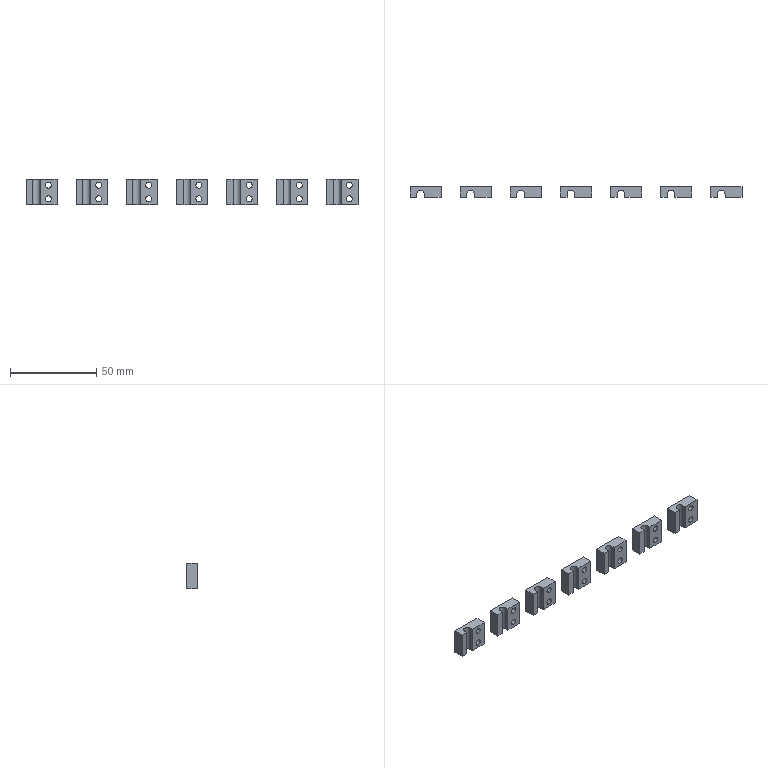NC program | Mastercam | posted with a generic post | part box 192 x 6 x 15 mm
Lines 2657 to 3876 of 12453:
(2 FEM |TOOL - 2|DIA. OFF. - 2|LEN. - 2|TOOL DIA. - 2.)
N5382 T2 M6
N5384 G0 G54 G90 X-65. Y1.856 C0. B0. S7000 M3
N5386 G43 H2 Z50.
N5388 Z3.61
N5390 G1 Z3.11 F600.
N5392 X-64.989 Z2.901 F3000.
N5394 X-64.957 Z2.694
N5396 X-64.902 Z2.492
N5398 X-64.827 Z2.296
N5400 X-64.732 Z2.11
N5402 X-64.618 Z1.934
N5404 X-64.487 Z1.771
N5406 X-64.338 Z1.623
N5408 X-64.176 Z1.492
N5410 X-64. Z1.378
N5412 X-63.814 Z1.283
N5414 X-63.618 Z1.208
N5416 X-63.416 Z1.153
N5418 X-63.209 Z1.121
N5420 X-63. Z1.11
N5422 G2 X-61. Y-.144 Z1. J-2.
N5424 G1 Y-1.244 Z.981
N5426 Y-2.344 Z.962
N5428 Y-3.444 Z.943
N5430 Y-4.544 Z.924
N5432 Y-6.4 Z.905
N5434 Y-5.644
N5436 Y-4.544 Z.886
N5438 Y-3.444 Z.867
N5440 Y-2.344 Z.848
N5442 Y-1.244 Z.83
N5444 Y-.144 Z.811
N5446 Y0. Z.808
N5448 Y.956 Z.792
N5450 Y2.056 Z.773
N5452 Y3.156 Z.754
N5454 Y4.256 Z.735
N5456 Y6.4 Z.716
N5458 Y5.356
N5460 Y4.256 Z.697
N5462 Y3.156 Z.678
N5464 Y2.056 Z.659
N5466 Y.956 Z.64
N5468 Y-.144 Z.621
N5470 Y-1.244 Z.602
N5472 Y-2.344 Z.583
N5474 Y-3.444 Z.564
N5476 Y-4.544 Z.545
N5478 Y-6.4 Z.527
N5480 Y-5.644
N5482 Y-4.544 Z.508
N5484 Y-3.444 Z.489
N5486 Y-2.344 Z.47
N5488 Y-1.244 Z.451
N5490 Y-.144 Z.432
N5492 Y0. Z.429
N5494 Y.956 Z.413
N5496 Y2.056 Z.394
N5498 Y3.156 Z.375
N5500 Y4.256 Z.356
N5502 Y6.4 Z.337
N5504 Y5.356
N5506 Y4.256 Z.318
N5508 Y3.156 Z.299
N5510 Y2.056 Z.28
N5512 Y.956 Z.261
N5514 Y-.144 Z.242
N5516 Y-1.244 Z.223
N5518 Y-2.344 Z.205
N5520 Y-3.444 Z.186
N5522 Y-4.544 Z.167
N5524 Y-6.4 Z.148
N5526 Y-5.644
N5528 Y-4.544 Z.129
N5530 Y-3.444 Z.11
N5532 Y-2.344 Z.091
N5534 Y-1.244 Z.072
N5536 Y-.144 Z.053
N5538 Y0. Z.051
N5540 Y.956 Z.034
N5542 Y2.056 Z.015
N5544 Y3.156 Z-.004
N5546 Y4.256 Z-.023
N5548 Y6.4 Z-.042
N5550 Y5.356
N5552 Y4.256 Z-.061
N5554 Y3.156 Z-.08
N5556 Y2.056 Z-.098
N5558 Y.956 Z-.117
N5560 Y-.144 Z-.136
N5562 Y-1.244 Z-.155
N5564 Y-2.344 Z-.174
N5566 Y-3.444 Z-.193
N5568 Y-4.544 Z-.212
N5570 Y-6.4 Z-.231
N5572 Y-5.644
N5574 Y-4.544 Z-.25
N5576 Y0.
N5578 Y6.4
N5580 Y-6.4
N5582 Y-4.544
N5584 G2 X-60.849 Y-4.346 I.206
N5586 G1 X-60.051 Y-4.124
N5588 G3 X-59.9 Y-3.926 I-.055 J.198
N5590 G1 Y0.
N5592 Y7.5
N5594 X-62.1
N5596 Y-7.5
N5598 X-59.9
N5600 Y-3.926
N5602 G3 X-59.902 Y-3.894 I-.206
N5604 G1 X-60.997 Y3.262
N5606 G2 X-61. Y3.293 I.203 J.031
N5608 G1 Y4.393 Z-.268
N5610 Y6.4 Z-.286
N5612 Y5.493
N5614 Y4.393 Z-.304
N5616 Y3.293 Z-.321
N5618 Y2.193 Z-.339
N5620 Y1.093 Z-.357
N5622 Y-.007 Z-.375
N5624 Y-1.107 Z-.393
N5626 Y-2.207 Z-.411
N5628 Y-3.307 Z-.429
N5630 Y-4.407 Z-.446
N5632 Y-6.4 Z-.464
N5634 Y-5.507
N5636 Y-4.407 Z-.482
N5638 Y-3.307 Z-.5
N5640 Y0.
N5642 Y6.4
N5644 Y-6.4
N5646 Y-3.307
N5648 G2 X-60.849 Y-3.108 I.206
N5650 G1 X-60.051 Y-2.887
N5652 G3 X-59.9 Y-2.688 I-.055 J.199
N5654 G1 Y0.
N5656 Y7.5
N5658 X-62.1
N5660 Y-7.5
N5662 X-59.9
N5664 Y-2.688
N5666 G3 X-59.902 Y-2.657 I-.206
N5668 G1 X-60.997 Y4.499
N5670 G2 X-61. Y4.531 I.203 J.032
N5672 G1 Y6.4 Z-.518
N5674 Y5.631
N5676 Y4.531 Z-.536
N5678 Y3.431 Z-.554
N5680 Y2.331 Z-.571
N5682 Y1.231 Z-.589
N5684 Y.131 Z-.607
N5686 Y-.969 Z-.625
N5688 Y-2.069 Z-.643
N5690 Y-3.169 Z-.661
N5692 Y-4.269 Z-.679
N5694 Y-6.4 Z-.696
N5696 Y-5.369
N5698 Y-4.269 Z-.714
N5700 Y-3.169 Z-.732
N5702 Y-2.069 Z-.75
N5704 Y0.
N5706 Y6.4
N5708 Y-6.4
N5710 Y-2.069
N5712 G2 X-60.849 Y-1.871 I.206
N5714 G1 X-60.051 Y-1.649
N5716 G3 X-59.9 Y-1.451 I-.055 J.198
N5718 G1 Y0.
N5720 Y7.5
N5722 X-62.1
N5724 Y-7.5
N5726 X-59.9
N5728 Y-1.451
N5730 G3 X-59.902 Y-1.423 I-.206
N5732 G1 X-60.59 Y3.596
N5734 G3 X-60.794 Y3.774 I-.204 J-.028
N5736 X-61. Y3.568 J-.206
N5738 G1 Y2.468 Z-.768
N5740 Y1.368 Z-.786
N5742 Y.268 Z-.804
N5744 Y-.832 Z-.821
N5746 Y-1.932 Z-.839
N5748 Y-3.032 Z-.857
N5750 Y-4.132 Z-.875
N5752 Y-5.232 Z-.893
N5754 Y-6.4 Z-.911
N5756 Y-6.332
N5758 Y-5.232 Z-.929
N5760 Y-4.132 Z-.946
N5762 Y-3.032 Z-.964
N5764 Y-1.932 Z-.982
N5766 Y-.832 Z-1.
N5768 Y0.
N5770 Y6.4
N5772 Y-6.4
N5774 Y-.832
N5776 G2 X-60.849 Y-.633 I.206
N5778 G1 X-60.051 Y-.412
N5780 G3 X-59.9 Y-.213 I-.055 J.199
N5782 G1 Y0.
N5784 Y7.5
N5786 X-62.1
N5788 Y-7.5
N5790 X-59.9
N5792 Y-.213
N5794 G3 X-59.902 Y-.183 I-.206
N5796 G1 X-60.59 Y4.43
N5798 G3 X-60.794 Y4.606 I-.204 J-.03
N5800 X-61. Y4.4 J-.206
N5802 G1 Y3.3 Z-1.018
N5804 Y2.2 Z-1.036
N5806 Y1.1 Z-1.054
N5808 Y0. Z-1.071
N5810 Y-1.1 Z-1.089
N5812 Y-2.2 Z-1.107
N5814 Y-3.3 Z-1.125
N5816 Y-4.4 Z-1.143
N5818 Y-6.4 Z-1.161
N5820 Y-5.5
N5822 Y-4.4 Z-1.179
N5824 Y-3.3 Z-1.196
N5826 Y-2.2 Z-1.214
N5828 Y-1.1 Z-1.232
N5830 Y0. Z-1.25
N5832 Y6.4
N5834 Y-6.4
N5836 Y0.
N5838 G2 X-60.849 Y.199 I.206
N5840 G1 X-60.051 Y.42
N5842 G3 X-59.9 Y.619 I-.055 J.199
N5844 G1 Y7.5
N5846 X-62.1
N5848 Y-7.5
N5850 X-59.9
N5852 Y0.
N5854 Y.619
N5856 G3 X-59.906 Y.668 I-.206
N5858 G1 X-60.594 Y3.486
N5860 G3 X-60.794 Y3.643 I-.2 J-.049
N5862 X-61. Y3.437 J-.206
N5864 G1 Y2.337 Z-1.268
N5866 Y1.237 Z-1.286
N5868 Y.137 Z-1.304
N5870 Y-.963 Z-1.321
N5872 Y-2.063 Z-1.339
N5874 Y-3.163 Z-1.357
N5876 Y-4.263 Z-1.375
N5878 Y-6.4 Z-1.393
N5880 Y-5.362
N5882 Y-4.263 Z-1.411
N5884 Y-3.163 Z-1.429
N5886 Y-2.063 Z-1.446
N5888 Y-.963 Z-1.464
N5890 Y0. Z-1.48
N5892 Y.138 Z-1.482
N5894 Y1.238 Z-1.5
N5896 Y6.4
N5898 Y-6.4
N5900 Y0.
N5902 Y1.238
N5904 G2 X-60.849 Y1.436 I.206
N5906 G1 X-60.051 Y1.657
N5908 G3 X-59.9 Y1.856 I-.055 J.199
N5910 G1 Y7.5
N5912 X-62.1
N5914 Y-7.5
N5916 X-59.9
N5918 Y0.
N5920 Y1.856
N5922 G3 X-60.106 Y2.062 I-.206
N5924 X-60.295 Y1.939 J-.206
N5926 G1 X-60.983 Y.357
N5928 G3 X-61. Y.275 I.189 J-.082
N5930 G1 Y-.825 Z-1.518
N5932 Y-1.925 Z-1.536
N5934 Y-3.025 Z-1.554
N5936 Y-4.125 Z-1.571
N5938 Y-5.225 Z-1.589
N5940 Y-6.4 Z-1.607
N5942 Y-6.325
N5944 Y-5.225 Z-1.625
N5946 Y-4.125 Z-1.643
N5948 Y-3.025 Z-1.661
N5950 Y-1.925 Z-1.679
N5952 Y-.825 Z-1.696
N5954 Y0. Z-1.71
N5956 Y.275 Z-1.714
N5958 Y1.375 Z-1.732
N5960 Y2.475 Z-1.75
N5962 Y6.4
N5964 Y-6.4
N5966 Y0.
N5968 Y2.475
N5970 G2 X-60.849 Y2.674 I.206
N5972 G1 X-60.051 Y2.895
N5974 G3 X-59.9 Y3.094 I-.055 J.199
N5976 G1 Y7.5
N5978 X-62.1
N5980 Y-7.5
N5982 X-59.9
N5984 Y0.
N5986 Y3.094
N5988 G3 X-60.106 Y3.3 I-.206
N5990 X-60.309 Y3.131 J-.206
N5992 G1 X-60.997 Y-.651
N5994 G3 X-61. Y-.688 I.203 J-.037
N5996 G1 Y-1.788 Z-1.768
N5998 Y-2.888 Z-1.786
N6000 Y-3.988 Z-1.804
N6002 Y-5.088 Z-1.821
N6004 Y-6.42 Z-1.839
N6006 Y-6.188
N6008 Y-5.088 Z-1.857
N6010 Y-3.988 Z-1.875
N6012 Y-2.888 Z-1.893
N6014 Y-1.788 Z-1.911
N6016 Y-.688 Z-1.929
N6018 Y.412 Z-1.946
N6020 Y1.512 Z-1.964
N6022 Y2.612 Z-1.982
N6024 Y3.712 Z-2.
N6026 Y6.42
N6028 Y0.
N6030 Y-6.42
N6032 Y3.712
N6034 G2 X-60.85 Y3.911 I.206
N6036 G1 X-60.07 Y4.133
N6038 G3 X-59.92 Y4.331 I-.056 J.198
N6040 G1 Y7.5
N6042 X-62.08
N6044 Y0.
N6046 Y-7.5
N6048 X-59.92
N6050 Y4.331
N6052 G3 X-60.126 Y4.537 I-.206
N6054 X-60.331 Y4.354 J-.206
N6056 G1 X-60.999 Y-1.627
N6058 G3 X-61. Y-1.65 I.205 J-.023
N6060 G1 Y-2.75 Z-2.018
N6062 Y-3.85 Z-2.036
N6064 Y-4.95 Z-2.054
N6066 Y-6.453 Z-2.071
N6068 Y-6.05
N6070 Y-4.95 Z-2.089
N6072 Y-3.85 Z-2.107
N6074 Y-2.75 Z-2.125
N6076 Y-1.65 Z-2.143
N6078 Y-.55 Z-2.161
N6080 Y0. Z-2.17
N6082 Y.55 Z-2.179
N6084 Y1.65 Z-2.196
N6086 Y2.75 Z-2.214
N6088 Y3.85 Z-2.232
N6090 Y4.95 Z-2.25
N6092 Y6.453
N6094 Y-6.453
N6096 Y0.
N6098 Y4.95
N6100 G2 X-60.852 Y5.148 I.206
N6102 G1 X-60.101 Y5.371
N6104 G3 X-59.953 Y5.569 I-.058 J.198
N6106 G1 Y7.5
N6108 X-62.047
N6110 Y-7.5
N6112 X-59.953
N6114 Y0.
N6116 Y5.569
N6118 G3 X-60.151 Y5.775 I-.206
N6120 G1 X-60.159
N6122 G3 X-60.365 Y5.585 J-.206
N6124 G1 X-61. Y-2.597
N6126 Y-2.613
N6128 Y-3.713 Z-2.268
N6130 Y-4.813 Z-2.286
N6132 Y-6.529 Z-2.304
N6134 Y-5.913
N6136 Y-4.813 Z-2.321
N6138 Y-3.713 Z-2.339
N6140 Y-2.613 Z-2.357
N6142 Y-1.513 Z-2.375
N6144 Y-.413 Z-2.393
N6146 Y0. Z-2.4
N6148 Y.687 Z-2.411
N6150 Y1.787 Z-2.429
N6152 Y2.887 Z-2.446
N6154 Y3.987 Z-2.464
N6156 Y5.087 Z-2.482
N6158 Y6.187 Z-2.5
N6160 Y6.529
N6162 Y-6.529
N6164 Y0.
N6166 Y6.187
N6168 G2 X-60.858 Y6.383 I.206
N6170 G1 X-60.17 Y6.61
N6172 G3 X-60.029 Y6.806 I-.065 J.196
N6174 G1 Y7.5
N6176 X-61.971
N6178 Y-7.5
N6180 X-60.029
N6182 Y0.
N6184 Y6.806
N6186 G3 X-60.128 Y6.909 I-.103
N6188 G1 X-60.132
N6190 G3 X-60.235 Y6.814 J-.103
N6192 G1 X-61. Y-2.763
N6194 Y-2.779
N6196 Y-3.879 Z-2.518
N6198 Y-4.979 Z-2.536
N6200 Y-6.639 Z-2.554
N6202 Y-6.079
N6204 Y-4.979 Z-2.571
N6206 Y-3.879 Z-2.589
N6208 Y-2.779 Z-2.607
N6210 Y-1.679 Z-2.625
N6212 Y-.579 Z-2.643
N6214 Y0. Z-2.652
N6216 Y.521 Z-2.661
N6218 Y1.621 Z-2.679
N6220 Y2.721 Z-2.696
N6222 Y3.821 Z-2.714
N6224 Y4.921 Z-2.732
N6226 Y6.639 Z-2.75
N6228 Y6.021
N6230 Y-6.639
N6232 Y0.
N6234 Y6.639
N6236 Y6.021
N6238 G2 X-61.131 Y5.828 I-.206
N6240 G1 X-61.73 Y5.594
N6242 G3 X-61.861 Y5.402 I.075 J-.192
N6244 G1 Y-7.5
N6246 X-60.139
N6248 Y0.
N6250 Y7.5
N6252 X-61.861
N6254 Y5.402
N6256 Y5.193 Z-2.739
N6258 Y4.986 Z-2.706
N6260 Y4.784 Z-2.652
N6262 Y4.588 Z-2.577
N6264 Y4.402 Z-2.482
N6266 Y4.226 Z-2.368
N6268 Y4.064 Z-2.236
N6270 Y3.916 Z-2.088
N6272 Y3.784 Z-1.926
N6274 Y3.67 Z-1.75
N6276 Y3.575 Z-1.563
N6278 Y3.5 Z-1.368
N6280 Y3.445 Z-1.166
N6282 Y3.413 Z-.959
N6284 Y3.402 Z-.75
N6286 Z-.25
N6288 G0 Z50.
N6290 X-60.282 Y-6.465
N6292 Z-.25
N6294 G1 Z-.75 F600.
N6296 Y-6.454 Z-.957 F3000.
N6298 Y-6.422 Z-1.162
N6300 Y-6.369 Z-1.362
N6302 Y-6.296 Z-1.556
N6304 Y-6.202 Z-1.741
N6306 Y-6.091 Z-1.915
N6308 Y-5.961 Z-2.077
N6310 Y-5.816 Z-2.225
N6312 Y-5.656 Z-2.357
N6314 Y-5.484 Z-2.471
N6316 Y-5.3 Z-2.568
N6318 Y-5.108 Z-2.644
N6320 Y-4.908 Z-2.701
N6322 Y-4.704 Z-2.736
N6324 Y-4.498 Z-2.75
N6326 Y-3.398 Z-2.768
N6328 Y-2.298 Z-2.786
N6330 Y-1.198 Z-2.804
N6332 Y-.098 Z-2.821
N6334 Y1.002 Z-2.839
N6336 Y2.102 Z-2.857
N6338 Y3.202 Z-2.875
N6340 Y4.302 Z-2.893
N6342 Y5.402 Z-2.911
N6344 Y6.502 Z-2.929
N6346 Y7.5 Z-2.945
N6348 X-60.747 Z-2.946
N6350 X-61.718 Z-2.962
N6352 Y6.983 Z-2.964
N6354 Y5.883 Z-2.982
N6356 Y4.783 Z-3.
N6358 Y0.
N6360 Y-7.5
N6362 X-60.282
N6364 Y7.5
N6366 X-61.718
N6368 Y4.783
N6370 G3 X-61.717 Y4.764 I.206
N6372 G1 X-60.899 Y-3.952
N6374 G3 X-60.693 Y-4.139 I.206 J.02
N6376 G1 X-60.684
N6378 G3 X-60.487 Y-3.932 I-.009 J.206
N6380 G1 Y-2.832 Z-3.018
N6382 Y-1.732 Z-3.036
N6384 Y-.632 Z-3.054
N6386 Y.468 Z-3.071
N6388 Y1.568 Z-3.089
N6390 Y2.668 Z-3.107
N6392 Y3.768 Z-3.125
N6394 Y4.868 Z-3.143
N6396 Y5.968 Z-3.161
N6398 Y7.068 Z-3.179
N6400 Y7.5 Z-3.186
N6402 X-61.513 Z-3.196
N6404 Y7.464
N6406 Y6.364 Z-3.214
N6408 Y5.264 Z-3.232
N6410 Y4.164 Z-3.25
N6412 Y0.
N6414 Y-7.5
N6416 X-60.487
N6418 Y7.5
N6420 X-61.513
N6422 Y4.164
N6424 Y4.157
N6426 X-61.19 Y-5.168
N6428 G3 X-60.984 Y-5.367 I.206 J.007
N6430 G1 X-60.98
N6432 G3 X-60.778 Y-5.161 I-.004 J.206
N6434 G1 Y-4.061 Z-3.268
N6436 Y-2.961 Z-3.286
N6438 Y-1.861 Z-3.304
N6440 Y-.761 Z-3.321
N6442 Y0. Z-3.334
N6444 Y.339 Z-3.339
N6446 Y1.439 Z-3.357
N6448 Y2.539 Z-3.375
N6450 Y3.639 Z-3.393
N6452 Y4.739 Z-3.411
N6454 Y5.839 Z-3.429
N6456 Y7.5 Z-3.446
N6458 X-61.222
N6460 Y6.846
N6462 Y5.746 Z-3.464
N6464 Y4.646 Z-3.482
N6466 Y3.546 Z-3.5
N6468 Y-7.443
N6470 Y-7.5
N6472 X-60.778
N6474 Y0.
N6476 Y7.5
N6478 X-61.222
N6480 Y3.546
N6482 Y3.336 Z-3.489
N6484 Y3.13 Z-3.456
N6486 Y2.928 Z-3.402
N6488 Y2.732 Z-3.327
N6490 Y2.546 Z-3.232
N6492 Y2.37 Z-3.118
N6494 Y2.207 Z-2.986
N6496 Y2.059 Z-2.838
N6498 Y1.928 Z-2.676
N6500 Y1.813 Z-2.5
N6502 Y1.718 Z-2.313
N6504 Y1.643 Z-2.118
N6506 Y1.589 Z-1.916
N6508 Y1.557 Z-1.709
N6510 Y1.546 Z-1.5
N6512 Z-1.
N6514 G0 Z50.
N6516 X-36. Y1.856
N6518 Z3.61
N6520 G1 Z3.11 F600.
N6522 X-35.989 Z2.901 F3000.
N6524 X-35.957 Z2.694
N6526 X-35.902 Z2.492
N6528 X-35.827 Z2.296
N6530 X-35.732 Z2.11
N6532 X-35.618 Z1.934
N6534 X-35.487 Z1.771
N6536 X-35.338 Z1.623
N6538 X-35.176 Z1.492
N6540 X-35. Z1.378
N6542 X-34.814 Z1.283
N6544 X-34.618 Z1.208
N6546 X-34.416 Z1.153
N6548 X-34.209 Z1.121
N6550 X-34. Z1.11
N6552 G2 X-32. Y-.144 Z1. J-2.
N6554 G1 Y-1.244 Z.981
N6556 Y-2.344 Z.962
N6558 Y-3.444 Z.943
N6560 Y-4.544 Z.924
N6562 Y-6.4 Z.905
N6564 Y-5.644
N6566 Y-4.544 Z.886
N6568 Y-3.444 Z.867
N6570 Y-2.344 Z.848
N6572 Y-1.244 Z.83
N6574 Y-.144 Z.811
N6576 Y0. Z.808
N6578 Y.956 Z.792
N6580 Y2.056 Z.773
N6582 Y3.156 Z.754
N6584 Y4.256 Z.735
N6586 Y6.4 Z.716
N6588 Y5.356
N6590 Y4.256 Z.697
N6592 Y3.156 Z.678
N6594 Y2.056 Z.659
N6596 Y.956 Z.64
N6598 Y-.144 Z.621
N6600 Y-1.244 Z.602
N6602 Y-2.344 Z.583
N6604 Y-3.444 Z.564
N6606 Y-4.544 Z.545
N6608 Y-6.4 Z.527
N6610 Y-5.644
N6612 Y-4.544 Z.508
N6614 Y-3.444 Z.489
N6616 Y-2.344 Z.47
N6618 Y-1.244 Z.451
N6620 Y-.144 Z.432
N6622 Y0. Z.429
N6624 Y.956 Z.413
N6626 Y2.056 Z.394
N6628 Y3.156 Z.375
N6630 Y4.256 Z.356
N6632 Y6.4 Z.337
N6634 Y5.356
N6636 Y4.256 Z.318
N6638 Y3.156 Z.299
N6640 Y2.056 Z.28
N6642 Y.956 Z.261
N6644 Y-.144 Z.242
N6646 Y-1.244 Z.223
N6648 Y-2.344 Z.205
N6650 Y-3.444 Z.186
N6652 Y-4.544 Z.167
N6654 Y-6.4 Z.148
N6656 Y-5.644
N6658 Y-4.544 Z.129
N6660 Y-3.444 Z.11
N6662 Y-2.344 Z.091
N6664 Y-1.244 Z.072
N6666 Y-.144 Z.053
N6668 Y0. Z.051
N6670 Y.956 Z.034
N6672 Y2.056 Z.015
N6674 Y3.156 Z-.004
N6676 Y4.256 Z-.023
N6678 Y6.4 Z-.042
N6680 Y5.356
N6682 Y4.256 Z-.061
N6684 Y3.156 Z-.08
N6686 Y2.056 Z-.098
N6688 Y.956 Z-.117
N6690 Y-.144 Z-.136
N6692 Y-1.244 Z-.155
N6694 Y-2.344 Z-.174
N6696 Y-3.444 Z-.193
N6698 Y-4.544 Z-.212
N6700 Y-6.4 Z-.231
N6702 Y-5.644
N6704 Y-4.544 Z-.25
N6706 Y0.
N6708 Y6.4
N6710 Y-6.4
N6712 Y-4.544
N6714 G2 X-31.849 Y-4.346 I.206
N6716 G1 X-31.051 Y-4.124
N6718 G3 X-30.9 Y-3.926 I-.055 J.198
N6720 G1 Y0.
N6722 Y7.5
N6724 X-33.1
N6726 Y-7.5
N6728 X-30.9
N6730 Y-3.926
N6732 G3 X-30.902 Y-3.894 I-.206
N6734 G1 X-31.997 Y3.262
N6736 G2 X-32. Y3.293 I.203 J.031
N6738 G1 Y4.393 Z-.268
N6740 Y6.4 Z-.286
N6742 Y5.493
N6744 Y4.393 Z-.304
N6746 Y3.293 Z-.321
N6748 Y2.193 Z-.339
N6750 Y1.093 Z-.357
N6752 Y-.007 Z-.375
N6754 Y-1.107 Z-.393
N6756 Y-2.207 Z-.411
N6758 Y-3.307 Z-.429
N6760 Y-4.407 Z-.446
N6762 Y-6.4 Z-.464
N6764 Y-5.507
N6766 Y-4.407 Z-.482
N6768 Y-3.307 Z-.5
N6770 Y0.
N6772 Y6.4
N6774 Y-6.4
N6776 Y-3.307
N6778 G2 X-31.849 Y-3.108 I.206
N6780 G1 X-31.051 Y-2.887
N6782 G3 X-30.9 Y-2.688 I-.055 J.199
N6784 G1 Y0.
N6786 Y7.5
N6788 X-33.1
N6790 Y-7.5
N6792 X-30.9
N6794 Y-2.688
N6796 G3 X-30.902 Y-2.657 I-.206
N6798 G1 X-31.997 Y4.499
N6800 G2 X-32. Y4.531 I.203 J.032
N6802 G1 Y6.4 Z-.518
N6804 Y5.631
N6806 Y4.531 Z-.536
N6808 Y3.431 Z-.554
N6810 Y2.331 Z-.571
N6812 Y1.231 Z-.589
N6814 Y.131 Z-.607
N6816 Y-.969 Z-.625
N6818 Y-2.069 Z-.643
N6820 Y-3.169 Z-.661
N6822 Y-4.269 Z-.679
N6824 Y-6.4 Z-.696
N6826 Y-5.369
N6828 Y-4.269 Z-.714
N6830 Y-3.169 Z-.732
N6832 Y-2.069 Z-.75
N6834 Y0.
N6836 Y6.4
N6838 Y-6.4
N6840 Y-2.069
N6842 G2 X-31.849 Y-1.871 I.206
N6844 G1 X-31.051 Y-1.649
N6846 G3 X-30.9 Y-1.451 I-.055 J.198
N6848 G1 Y0.
N6850 Y7.5
N6852 X-33.1
N6854 Y-7.5
N6856 X-30.9
N6858 Y-1.451
N6860 G3 X-30.902 Y-1.423 I-.206
N6862 G1 X-31.59 Y3.596
N6864 G3 X-31.794 Y3.774 I-.204 J-.028
N6866 X-32. Y3.568 J-.206
N6868 G1 Y2.468 Z-.768
N6870 Y1.368 Z-.786
N6872 Y.268 Z-.804
N6874 Y-.832 Z-.821
N6876 Y-1.932 Z-.839
N6878 Y-3.032 Z-.857
N6880 Y-4.132 Z-.875
N6882 Y-5.232 Z-.893
N6884 Y-6.4 Z-.911
N6886 Y-6.332
N6888 Y-5.232 Z-.929
N6890 Y-4.132 Z-.946
N6892 Y-3.032 Z-.964
N6894 Y-1.932 Z-.982
N6896 Y-.832 Z-1.
N6898 Y0.
N6900 Y6.4
N6902 Y-6.4
N6904 Y-.832
N6906 G2 X-31.849 Y-.633 I.206
N6908 G1 X-31.051 Y-.412
N6910 G3 X-30.9 Y-.213 I-.055 J.199
N6912 G1 Y0.
N6914 Y7.5
N6916 X-33.1
N6918 Y-7.5
N6920 X-30.9
N6922 Y-.213
N6924 G3 X-30.902 Y-.183 I-.206
N6926 G1 X-31.59 Y4.43
N6928 G3 X-31.794 Y4.606 I-.204 J-.03
N6930 X-32. Y4.4 J-.206
N6932 G1 Y3.3 Z-1.018
N6934 Y2.2 Z-1.036
N6936 Y1.1 Z-1.054
N6938 Y0. Z-1.071
N6940 Y-1.1 Z-1.089
N6942 Y-2.2 Z-1.107
N6944 Y-3.3 Z-1.125
N6946 Y-4.4 Z-1.143
N6948 Y-6.4 Z-1.161
N6950 Y-5.5
N6952 Y-4.4 Z-1.179
N6954 Y-3.3 Z-1.196
N6956 Y-2.2 Z-1.214
N6958 Y-1.1 Z-1.232
N6960 Y0. Z-1.25
N6962 Y6.4
N6964 Y-6.4
N6966 Y0.
N6968 G2 X-31.849 Y.199 I.206
N6970 G1 X-31.051 Y.42
N6972 G3 X-30.9 Y.619 I-.055 J.199
N6974 G1 Y7.5
N6976 X-33.1
N6978 Y-7.5
N6980 X-30.9
N6982 Y0.
N6984 Y.619
N6986 G3 X-30.906 Y.668 I-.206
N6988 G1 X-31.594 Y3.486
N6990 G3 X-31.794 Y3.643 I-.2 J-.049
N6992 X-32. Y3.437 J-.206
N6994 G1 Y2.337 Z-1.268
N6996 Y1.237 Z-1.286
N6998 Y.137 Z-1.304
N7000 Y-.963 Z-1.321
N7002 Y-2.063 Z-1.339
N7004 Y-3.163 Z-1.357
N7006 Y-4.263 Z-1.375
N7008 Y-6.4 Z-1.393
N7010 Y-5.362
N7012 Y-4.263 Z-1.411
N7014 Y-3.163 Z-1.429
N7016 Y-2.063 Z-1.446
N7018 Y-.963 Z-1.464
N7020 Y0. Z-1.48
N7022 Y.138 Z-1.482
N7024 Y1.238 Z-1.5
N7026 Y6.4
N7028 Y-6.4
N7030 Y0.
N7032 Y1.238
N7034 G2 X-31.849 Y1.436 I.206
N7036 G1 X-31.051 Y1.657
N7038 G3 X-30.9 Y1.856 I-.055 J.199
N7040 G1 Y7.5
N7042 X-33.1
N7044 Y-7.5
N7046 X-30.9
N7048 Y0.
N7050 Y1.856
N7052 G3 X-31.106 Y2.062 I-.206
N7054 X-31.295 Y1.939 J-.206
N7056 G1 X-31.983 Y.357
N7058 G3 X-32. Y.275 I.189 J-.082
N7060 G1 Y-.825 Z-1.518
N7062 Y-1.925 Z-1.536
N7064 Y-3.025 Z-1.554
N7066 Y-4.125 Z-1.571
N7068 Y-5.225 Z-1.589
N7070 Y-6.4 Z-1.607
N7072 Y-6.325
N7074 Y-5.225 Z-1.625
N7076 Y-4.125 Z-1.643
N7078 Y-3.025 Z-1.661
N7080 Y-1.925 Z-1.679
N7082 Y-.825 Z-1.696
N7084 Y0. Z-1.71
N7086 Y.275 Z-1.714
N7088 Y1.375 Z-1.732
N7090 Y2.475 Z-1.75
N7092 Y6.4
N7094 Y-6.4
N7096 Y0.
N7098 Y2.475
N7100 G2 X-31.849 Y2.674 I.206
N7102 G1 X-31.051 Y2.895
N7104 G3 X-30.9 Y3.094 I-.055 J.199
N7106 G1 Y7.5
N7108 X-33.1
N7110 Y-7.5
N7112 X-30.9
N7114 Y0.
N7116 Y3.094
N7118 G3 X-31.106 Y3.3 I-.206
N7120 X-31.309 Y3.131 J-.206
N7122 G1 X-31.997 Y-.651
N7124 G3 X-32. Y-.688 I.203 J-.037
N7126 G1 Y-1.788 Z-1.768
N7128 Y-2.888 Z-1.786
N7130 Y-3.988 Z-1.804
N7132 Y-5.088 Z-1.821
N7134 Y-6.42 Z-1.839
N7136 Y-6.188
N7138 Y-5.088 Z-1.857
N7140 Y-3.988 Z-1.875
N7142 Y-2.888 Z-1.893
N7144 Y-1.788 Z-1.911
N7146 Y-.688 Z-1.929
N7148 Y.412 Z-1.946
N7150 Y1.512 Z-1.964
N7152 Y2.612 Z-1.982
N7154 Y3.712 Z-2.
N7156 Y6.42
N7158 Y0.
N7160 Y-6.42
N7162 Y3.712
N7164 G2 X-31.85 Y3.911 I.206
N7166 G1 X-31.07 Y4.133
N7168 G3 X-30.92 Y4.331 I-.056 J.198
N7170 G1 Y7.5
N7172 X-33.08
N7174 Y0.
N7176 Y-7.5
N7178 X-30.92
N7180 Y4.331
N7182 G3 X-31.126 Y4.537 I-.206
N7184 X-31.331 Y4.354 J-.206
N7186 G1 X-31.999 Y-1.627
N7188 G3 X-32. Y-1.65 I.205 J-.023
N7190 G1 Y-2.75 Z-2.018
N7192 Y-3.85 Z-2.036
N7194 Y-4.95 Z-2.054
N7196 Y-6.453 Z-2.071
N7198 Y-6.05
N7200 Y-4.95 Z-2.089
N7202 Y-3.85 Z-2.107
N7204 Y-2.75 Z-2.125
N7206 Y-1.65 Z-2.143
N7208 Y-.55 Z-2.161
N7210 Y0. Z-2.17
N7212 Y.55 Z-2.179
N7214 Y1.65 Z-2.196
N7216 Y2.75 Z-2.214
N7218 Y3.85 Z-2.232
N7220 Y4.95 Z-2.25
N7222 Y6.453
N7224 Y-6.453
N7226 Y0.
N7228 Y4.95
N7230 G2 X-31.852 Y5.148 I.206
N7232 G1 X-31.101 Y5.371
N7234 G3 X-30.953 Y5.569 I-.058 J.198
N7236 G1 Y7.5
N7238 X-33.047
N7240 Y-7.5
N7242 X-30.953
N7244 Y0.
N7246 Y5.569
N7248 G3 X-31.151 Y5.775 I-.206
N7250 G1 X-31.159
N7252 G3 X-31.365 Y5.585 J-.206
N7254 G1 X-32. Y-2.597
N7256 Y-2.613
N7258 Y-3.713 Z-2.268
N7260 Y-4.813 Z-2.286
N7262 Y-6.529 Z-2.304
N7264 Y-5.913
N7266 Y-4.813 Z-2.321
N7268 Y-3.713 Z-2.339
N7270 Y-2.613 Z-2.357
N7272 Y-1.513 Z-2.375
N7274 Y-.413 Z-2.393
N7276 Y0. Z-2.4
N7278 Y.687 Z-2.411
N7280 Y1.787 Z-2.429
N7282 Y2.887 Z-2.446
N7284 Y3.987 Z-2.464
N7286 Y5.087 Z-2.482
N7288 Y6.187 Z-2.5
N7290 Y6.529
N7292 Y-6.529
N7294 Y0.
N7296 Y6.187
N7298 G2 X-31.858 Y6.383 I.206
N7300 G1 X-31.17 Y6.61
N7302 G3 X-31.029 Y6.806 I-.065 J.196
N7304 G1 Y7.5
N7306 X-32.971
N7308 Y-7.5
N7310 X-31.029
N7312 Y0.
N7314 Y6.806
N7316 G3 X-31.128 Y6.909 I-.103
N7318 G1 X-31.132
N7320 G3 X-31.235 Y6.814 J-.103
N7322 G1 X-32. Y-2.763
N7324 Y-2.779
N7326 Y-3.879 Z-2.518
N7328 Y-4.979 Z-2.536
N7330 Y-6.639 Z-2.554
N7332 Y-6.079
N7334 Y-4.979 Z-2.571
N7336 Y-3.879 Z-2.589
N7338 Y-2.779 Z-2.607
N7340 Y-1.679 Z-2.625
N7342 Y-.579 Z-2.643
N7344 Y0. Z-2.652
N7346 Y.521 Z-2.661
N7348 Y1.621 Z-2.679
N7350 Y2.721 Z-2.696
N7352 Y3.821 Z-2.714
N7354 Y4.921 Z-2.732
N7356 Y6.639 Z-2.75
N7358 Y6.021
N7360 Y-6.639
N7362 Y0.
N7364 Y6.639
N7366 Y6.021
N7368 G2 X-32.131 Y5.828 I-.206
N7370 G1 X-32.73 Y5.594
N7372 G3 X-32.861 Y5.402 I.075 J-.192
N7374 G1 Y-7.5
N7376 X-31.139
N7378 Y0.
N7380 Y7.5
N7382 X-32.861
N7384 Y5.402
N7386 Y5.193 Z-2.739
N7388 Y4.986 Z-2.706
N7390 Y4.784 Z-2.652
N7392 Y4.588 Z-2.577
N7394 Y4.402 Z-2.482
N7396 Y4.226 Z-2.368
N7398 Y4.064 Z-2.236
N7400 Y3.916 Z-2.088
N7402 Y3.784 Z-1.926
N7404 Y3.67 Z-1.75
N7406 Y3.575 Z-1.563
N7408 Y3.5 Z-1.368
N7410 Y3.445 Z-1.166
N7412 Y3.413 Z-.959
N7414 Y3.402 Z-.75
N7416 Z-.25
N7418 G0 Z50.
N7420 X-31.282 Y-6.465
N7422 Z-.25
N7424 G1 Z-.75 F600.
N7426 Y-6.454 Z-.957 F3000.
N7428 Y-6.422 Z-1.162
N7430 Y-6.369 Z-1.362
N7432 Y-6.296 Z-1.556
N7434 Y-6.202 Z-1.741
N7436 Y-6.091 Z-1.915
N7438 Y-5.961 Z-2.077
N7440 Y-5.816 Z-2.225
N7442 Y-5.656 Z-2.357
N7444 Y-5.484 Z-2.471
N7446 Y-5.3 Z-2.568
N7448 Y-5.108 Z-2.644
N7450 Y-4.908 Z-2.701
N7452 Y-4.704 Z-2.736
N7454 Y-4.498 Z-2.75
N7456 Y-3.398 Z-2.768
N7458 Y-2.298 Z-2.786
N7460 Y-1.198 Z-2.804
N7462 Y-.098 Z-2.821
N7464 Y1.002 Z-2.839
N7466 Y2.102 Z-2.857
N7468 Y3.202 Z-2.875
N7470 Y4.302 Z-2.893
N7472 Y5.402 Z-2.911
N7474 Y6.502 Z-2.929
N7476 Y7.5 Z-2.945
N7478 X-31.747 Z-2.946
N7480 X-32.718 Z-2.962
N7482 Y6.983 Z-2.964
N7484 Y5.883 Z-2.982
N7486 Y4.783 Z-3.
N7488 Y0.
N7490 Y-7.5
N7492 X-31.282
N7494 Y7.5
N7496 X-32.718
N7498 Y4.783
N7500 G3 X-32.717 Y4.764 I.206
N7502 G1 X-31.899 Y-3.952
N7504 G3 X-31.693 Y-4.139 I.206 J.02
N7506 G1 X-31.684
N7508 G3 X-31.487 Y-3.932 I-.009 J.206
N7510 G1 Y-2.832 Z-3.018
N7512 Y-1.732 Z-3.036
N7514 Y-.632 Z-3.054
N7516 Y.468 Z-3.071
N7518 Y1.568 Z-3.089
N7520 Y2.668 Z-3.107
N7522 Y3.768 Z-3.125
N7524 Y4.868 Z-3.143
N7526 Y5.968 Z-3.161
N7528 Y7.068 Z-3.179
N7530 Y7.5 Z-3.186
N7532 X-32.513 Z-3.196
N7534 Y7.464
N7536 Y6.364 Z-3.214
N7538 Y5.264 Z-3.232
N7540 Y4.164 Z-3.25
N7542 Y0.
N7544 Y-7.5
N7546 X-31.487
N7548 Y7.5
N7550 X-32.513
N7552 Y4.164
N7554 Y4.157
N7556 X-32.19 Y-5.168
N7558 G3 X-31.984 Y-5.367 I.206 J.007
N7560 G1 X-31.98
N7562 G3 X-31.778 Y-5.161 I-.004 J.206
N7564 G1 Y-4.061 Z-3.268
N7566 Y-2.961 Z-3.286
N7568 Y-1.861 Z-3.304
N7570 Y-.761 Z-3.321
N7572 Y0. Z-3.334
N7574 Y.339 Z-3.339
N7576 Y1.439 Z-3.357
N7578 Y2.539 Z-3.375
N7580 Y3.639 Z-3.393
N7582 Y4.739 Z-3.411
N7584 Y5.839 Z-3.429
N7586 Y7.5 Z-3.446
N7588 X-32.222
N7590 Y6.846
N7592 Y5.746 Z-3.464
N7594 Y4.646 Z-3.482
N7596 Y3.546 Z-3.5
N7598 Y-7.443
N7600 Y-7.5
N7602 X-31.778
N7604 Y0.
N7606 Y7.5
N7608 X-32.222
N7610 Y3.546
N7612 Y3.336 Z-3.489
N7614 Y3.13 Z-3.456
N7616 Y2.928 Z-3.402
N7618 Y2.732 Z-3.327
N7620 Y2.546 Z-3.232
N7622 Y2.37 Z-3.118
N7624 Y2.207 Z-2.986
N7626 Y2.059 Z-2.838
N7628 Y1.928 Z-2.676
N7630 Y1.813 Z-2.5
N7632 Y1.718 Z-2.313
N7634 Y1.643 Z-2.118
N7636 Y1.589 Z-1.916
N7638 Y1.557 Z-1.709
N7640 Y1.546 Z-1.5
N7642 Z-1.
N7644 G0 Z50.
N7646 X-7. Y1.856
N7648 Z3.61
N7650 G1 Z3.11 F600.
N7652 X-6.989 Z2.901 F3000.
N7654 X-6.957 Z2.694
N7656 X-6.902 Z2.492
N7658 X-6.827 Z2.296
N7660 X-6.732 Z2.11
N7662 X-6.618 Z1.934
N7664 X-6.487 Z1.771
N7666 X-6.338 Z1.623
N7668 X-6.176 Z1.492
N7670 X-6. Z1.378
N7672 X-5.814 Z1.283
N7674 X-5.618 Z1.208
N7676 X-5.416 Z1.153
N7678 X-5.209 Z1.121
N7680 X-5. Z1.11
N7682 G2 X-3. Y-.144 Z1. J-2.
N7684 G1 Y-1.244 Z.981
N7686 Y-2.344 Z.962
N7688 Y-3.444 Z.943
N7690 Y-4.544 Z.924
N7692 Y-6.4 Z.905
N7694 Y-5.644
N7696 Y-4.544 Z.886
N7698 Y-3.444 Z.867
N7700 Y-2.344 Z.848
N7702 Y-1.244 Z.83
N7704 Y-.144 Z.811
N7706 Y0. Z.808
N7708 Y.956 Z.792
N7710 Y2.056 Z.773
N7712 Y3.156 Z.754
N7714 Y4.256 Z.735
N7716 Y6.4 Z.716
N7718 Y5.356
N7720 Y4.256 Z.697
N7722 Y3.156 Z.678
N7724 Y2.056 Z.659
N7726 Y.956 Z.64
N7728 Y-.144 Z.621
N7730 Y-1.244 Z.602
N7732 Y-2.344 Z.583
N7734 Y-3.444 Z.564
N7736 Y-4.544 Z.545
N7738 Y-6.4 Z.527
N7740 Y-5.644
N7742 Y-4.544 Z.508
N7744 Y-3.444 Z.489
N7746 Y-2.344 Z.47
N7748 Y-1.244 Z.451
N7750 Y-.144 Z.432
N7752 Y0. Z.429
N7754 Y.956 Z.413
N7756 Y2.056 Z.394
N7758 Y3.156 Z.375
N7760 Y4.256 Z.356
N7762 Y6.4 Z.337
N7764 Y5.356
N7766 Y4.256 Z.318
N7768 Y3.156 Z.299
N7770 Y2.056 Z.28
N7772 Y.956 Z.261
N7774 Y-.144 Z.242
N7776 Y-1.244 Z.223
N7778 Y-2.344 Z.205
N7780 Y-3.444 Z.186
N7782 Y-4.544 Z.167
N7784 Y-6.4 Z.148
N7786 Y-5.644
N7788 Y-4.544 Z.129
N7790 Y-3.444 Z.11
N7792 Y-2.344 Z.091
N7794 Y-1.244 Z.072
N7796 Y-.144 Z.053
N7798 Y0. Z.051
N7800 Y.956 Z.034
N7802 Y2.056 Z.015
N7804 Y3.156 Z-.004
N7806 Y4.256 Z-.023
N7808 Y6.4 Z-.042
N7810 Y5.356
N7812 Y4.256 Z-.061
N7814 Y3.156 Z-.08
N7816 Y2.056 Z-.098
N7818 Y.956 Z-.117